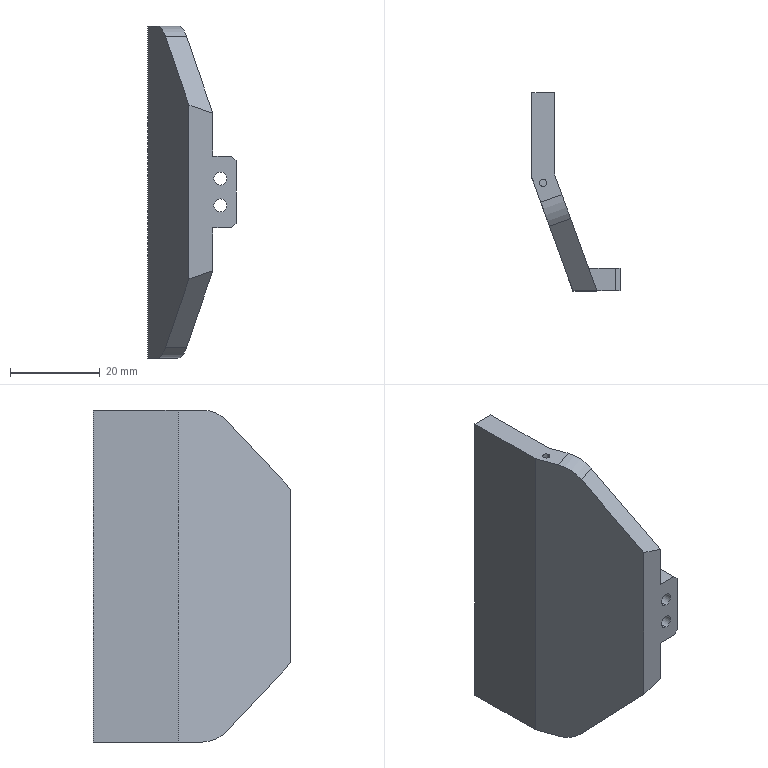NC program | NX | posted with a generic post | part box 19.643 x 44.061 x 74 mm
Lines 1 to 841 of 6515:
N10 G17 G21 G94 G90
(ADAPTIVE_MILLING_1 , TOOL : D8开粗)
N12 T02 M6
N14 G54
N16 G17 G0 G90 X47.519 Y39.467 B0. C0. S6500 M3
N18 G43 Z30. H2
N20 Z-18.35
N22 G94 G1 X47.451 Y39.6 Z-19.287 F3000.
N24 X47.383 Y39.734 Z-19.658
N26 X47.314 Y39.868 Z-19.93
N28 X47.246 Y40.001 Z-20.15
N30 X47.178 Y40.135 Z-20.334
N32 X47.109 Y40.268 Z-20.492
N34 X47.041 Y40.402 Z-20.63
N36 X46.972 Y40.535 Z-20.75
N38 X46.904 Y40.669 Z-20.855
N40 X46.836 Y40.802 Z-20.948
N42 X46.767 Y40.936 Z-21.029
N44 X46.699 Y41.069 Z-21.1
N46 X46.631 Y41.203 Z-21.16
N48 X46.562 Y41.336 Z-21.212
N50 X46.494 Y41.47 Z-21.255
N52 X46.426 Y41.603 Z-21.289
N54 X46.357 Y41.737 Z-21.316
N56 X46.289 Y41.87 Z-21.335
N58 X46.221 Y42.004 Z-21.346
N60 X46.152 Y42.138 Z-21.35
N62 X45.419 Y43.571
N64 G3 X43.987 Y43.584 R0.808
N66 G2 X43.689 Y42.483 R13.522
N68 G3 X43.278 Y38.319 R22.901
N70 X43.199 Y28.427 R395.024
N72 G1 X43.198 Y1.227
N74 G2 X41.595 Y-1.881 R4.329
N76 X37.82 Y-3.617 R8.394
N78 X32.452 Y-4.133 R29.955
N80 X22.352 Y-4.198 R519.939
N82 G1 X-37.82 Y-4.196
N84 G2 X-40.911 Y-2.558 R4.362
N86 X-42.627 Y1.228 R8.498
N88 X-43.134 Y6.597 R30.315
N90 X-43.199 Y16.596 R510.859
N92 G1 X-43.198 Y41.384
N94 G3 X-43.307 Y41.858 R1.202
N96 G1 X-43.582 Y42.28
N98 G2 X-43.965 Y43.549 R5.41
N100 G1 X-44.011 Y43.638
N102 G3 X-45.486 Y43.549 R0.808
N104 G1 X-45.765 Y42.801
N106 G3 X-45.725 Y42.146 R0.811
N108 G1 X-45.656 Y42.013 Z-21.346
N110 X-45.587 Y41.879 Z-21.335
N112 X-45.518 Y41.746 Z-21.316
N114 X-45.449 Y41.613 Z-21.289
N116 X-45.38 Y41.48 Z-21.255
N118 X-45.311 Y41.347 Z-21.212
N120 X-45.241 Y41.214 Z-21.16
N122 X-45.172 Y41.081 Z-21.1
N124 X-45.103 Y40.948 Z-21.029
N126 X-45.034 Y40.815 Z-20.948
N128 X-44.965 Y40.682 Z-20.855
N130 X-44.896 Y40.548 Z-20.75
N132 X-44.826 Y40.415 Z-20.63
N134 X-44.757 Y40.282 Z-20.492
N136 X-44.688 Y40.149 Z-20.334
N138 X-44.619 Y40.016 Z-20.15
N140 X-44.55 Y39.883 Z-19.93
N142 X-44.481 Y39.75 Z-19.658
N144 X-44.411 Y39.617 Z-19.287
N146 X-44.342 Y39.484 Z-18.35
N148 G0 Z30.
N150 X49.186 Y42.158
N152 Z-18.35
N154 G1 X49.036 Y42.157 Z-19.287
N156 X48.886 Y42.156 Z-19.658
N158 X48.736 Y42.155 Z-19.93
N160 X48.586 Y42.154 Z-20.15
N162 X48.436 Y42.153 Z-20.334
N164 X48.286 Y42.152 Z-20.492
N166 X48.136 Y42.151 Z-20.63
N168 X47.986 Y42.15 Z-20.75
N170 X47.836 Y42.149 Z-20.855
N172 X47.686 Y42.148 Z-20.948
N174 X47.536 Y42.147 Z-21.029
N176 X47.386 Y42.146 Z-21.1
N178 X47.236 Y42.145 Z-21.16
N180 X47.086 Y42.144 Z-21.212
N182 X46.936 Y42.143 Z-21.255
N184 X46.786 Y42.142 Z-21.289
N186 X46.636 Y42.141 Z-21.316
N188 X46.486 Y42.14 Z-21.335
N190 X46.336 Y42.139 Z-21.346
N192 X46.186 Y42.138 Z-21.35
N194 G2 X45.458 Y42.585 R0.809
N196 G1 X45.339 Y42.829
N198 X45.206 Y43.066
N200 G3 X43.792 Y42.864 R0.808
N202 G2 X43.35 Y41.852 R4.978
N204 G3 X42.658 Y38.601 R11.16
N206 X42.413 Y31.11 R91.281
N208 G1 X42.4 Y23.527
N210 X42.399 Y3.627
N212 G2 X39.878 Y-1.036 R5.88
N214 X35.46 Y-2.819 R10.805
N216 X29.489 Y-3.334 R37.58
N218 X21.889 Y-3.405 R624.145
N220 G3 X21.405 Y-3.619 R1.216
N222 G2 X19.349 Y-4.15 R4.218
N224 G1 X-19.35
N226 G2 X-20.963 Y-3.864 R6.112
N228 G3 X-25.268 Y-3.468 R24.879
N230 X-35.673 Y-3.385 R646.994
N232 G2 X-40.095 Y-0.795 R5.925
N234 X-41.819 Y3.542 R10.895
N236 X-42.339 Y9.713 R38.434
N238 X-42.398 Y20.113 R642.761
N240 G1 X-42.399 Y39.27
N242 G3 X-42.543 Y40.89 R5.724
N244 X-43.08 Y41.509 R2.07
N246 G1 X-43.352 Y41.928
N248 G3 X-44.446 Y42.171 R0.8
N250 X-44.827 Y41.505 Z-21.299 R0.832
N252 G1 X-44.914 Y40.737 Z-21.25
N254 X-45.121 Y38.865 F15000.
N256 Y11.851
N258 G3 X-44.506 Y5.031 R38.162
N260 G1 X-44.281 Y3.774
N262 X-44.038 Y2.522
N264 G3 X-42.742 Y-1.057 R14.501
N266 X-41.513 Y-2.978 R15.741
N268 X-40.029 Y-4.321 R5.81
N270 X-38.641 Y-5.034 R7.849
N272 X-36.99 Y-5.588 R11.3
N274 X-35.34 Y-5.823 R9.123
N276 G1 X-23.257 Y-6.413
N278 G3 X-22.886 Y-6.342 R0.84
N280 G1 X-21.535 Y-5.725
N282 X-21.089 Y-5.526 Z-21.281 F3000.
N284 X-20.65 Y-5.312 Z-21.312
N286 G3 X-20.312 Y-4.84 Z-21.35 R0.82
N288 X-20.756 Y-3.913 R0.8
N290 X-24.362 Y-2.902 R9.635
N292 X-31.396 Y-2.616 R73.042
N294 G2 X-34.381 Y-2.532 R27.551
N296 X-39.329 Y0.732 R6.952
N298 X-41.059 Y5.608 R12.894
N300 X-41.547 Y12.285 R47.439
N302 X-41.598 Y23.963 R752.767
N304 G1 X-41.599 Y37.464
N306 G3 X-41.764 Y39.951 R13.052
N308 X-42.415 Y40.872 R1.137
N310 G1 X-42.704 Y41.149
N312 G3 X-43.647 Y41.269 R0.8
N314 X-44.059 Y40.626 Z-21.3 R0.832
N316 G1 X-44.187 Y39.859 Z-21.25
N318 X-44.461 Y38.218 F15000.
N320 X-44.472 Y38.086
N322 Y16.966
N324 G3 X-43.847 Y8.17 R62.252
N326 G1 X-43.6 Y6.42
N328 X-43.337 Y4.672
N330 G3 X-42.42 Y1.478 R15.765
N332 X-41.535 Y-0.265 R13.083
N334 G1 X-41.071 Y-1.034
N336 X-40.594 Y-1.796
N338 G3 X-39.167 Y-3.193 R5.39
N340 X-37.794 Y-3.931 R7.292
N342 X-35.475 Y-4.691 R12.9
N344 X-33.784 Y-4.943 R16.452
N346 G1 X-32.686 Y-5.04
N348 X-31.586 Y-5.103
N350 X-24.47 Y-5.386
N352 X-24.347 Y-5.381
N354 X-22.622 Y-5.183
N356 X-22.129 Y-5.129 Z-21.282 F3000.
N358 X-21.639 Y-5.061 Z-21.313
N360 G3 X-21.177 Y-4.729 Z-21.35 R0.82
N362 X-21.408 Y-3.618 R0.8
N364 X-24.521 Y-2.342 R6.919
N366 X-30.258 Y-1.871 R38.181
N368 G2 X-33.43 Y-1.652 R18.825
N370 X-38.545 Y2.083 R7.687
N372 X-40.237 Y7.081 R14.105
N374 X-40.748 Y14.457 R51.567
N376 G1 X-40.782 Y16.924
N378 G2 X-41.15 Y19.692 R12.965
N380 G1 X-41.162 Y39.106
N382 G3 X-41.486 Y40.256 R2.241
N384 X-42.186 Y40.737 R2.579
N386 X-43.402 Y39.552 R0.88
N388 G1 X-42.8 Y38.466
N390 G3 X-41.15 Y38.892 R0.88
N392 X-41.174 Y39.802 R10.963
N394 X-41.738 Y40.473 R0.999
N396 X-42.541 Y40.479 R0.801
N398 X-42.884 Y40.125 Z-21.318 R1.067
N400 G1 X-43.509 Y39.252 Z-21.25
N402 X-44.089 Y38.444 F15000.
N404 G3 X-44.238 Y37.972 R0.81
N406 G1 X-44.218 Y34.372
N408 X-44.182 Y30.771
N410 G3 X-43.784 Y21.781 R167.581
N412 G1 X-42.839 Y8.553
N414 G3 X-42.083 Y4.147 R22.504
N416 X-40.552 Y0.638 R15.458
N418 X-38.707 Y-1.601 R8.256
N420 X-37.389 Y-2.616 R11.042
N422 X-34.887 Y-3.698 R8.477
N424 X-31.522 Y-4.34 R23.261
N426 G1 X-24.942 Y-5.078
N428 X-24.734 Y-5.074
N430 X-23.133 Y-4.834
N432 X-22.65 Y-4.765 Z-21.281 F3000.
N434 X-22.168 Y-4.68 Z-21.312
N436 G3 X-21.713 Y-4.32 Z-21.35 R0.82
N438 X-21.88 Y-3.31 R0.8
N440 X-24.557 Y-1.837 R5.524
N442 X-29.272 Y-1.184 R23.936
N444 G2 X-32.728 Y-0.745 R15.977
N446 X-37.791 Y3.379 R8.362
N448 X-39.464 Y8.697 R15.675
N450 X-39.912 Y14.476 R50.345
N452 G3 X-40.264 Y15.339 R4.186
N454 G2 X-40.786 Y16.945 R16.439
N456 G3 X-42.246 Y17.213 R0.8
N458 X-42.379 Y16.683 Z-21.315 R1.026
N460 G1 X-42.448 Y15.667 Z-21.25
N462 X-42.56 Y13.958 F15000.
N464 X-41.83 Y8.033
N466 G3 X-40.713 Y3.794 R16.281
N468 X-38.925 Y0.913 R11.255
N470 G1 X-38.185 Y0.043
N472 X-37.435 Y-0.818
N474 G3 X-36.179 Y-1.84 R6.318
N476 X-32.546 Y-3.249 R10.674
N478 G1 X-25.518 Y-4.57
N480 X-25.378 Y-4.581
N482 X-25.237 Y-4.572
N484 X-23.732 Y-4.318
N486 X-23.243 Y-4.239 Z-21.282 F3000.
N488 X-22.758 Y-4.145 Z-21.313
N490 G3 X-22.314 Y-3.789 Z-21.35 R0.82
N492 X-22.455 Y-2.801 R0.8
N494 X-25.136 Y-1.194 R5.529
N496 X-29.158 Y-0.477 R22.394
N498 G2 X-33.36 Y0.723 R11.126
N500 X-37.422 Y5.402 R9.596
N502 X-38.803 Y11.115 R19.758
N504 G3 X-39.012 Y13.042 R70.143
N506 X-39.529 Y13.873 R4.31
N508 G1 X-39.996 Y14.757
N510 G3 X-41.153 Y15.045 R0.8
N512 X-41.506 Y14.4 Z-21.302 R0.837
N514 G1 X-41.597 Y13.596 Z-21.25
N516 X-41.697 Y12.737 F15000.
N518 X-41.786 Y11.878
N520 X-41.764 Y11.694
N522 X-41.423 Y10.263
N524 X-41.053 Y8.84
N526 G3 X-40.003 Y5.496 R72.342
N528 X-38.576 Y2.468 R17.102
N530 G1 X-38.225 Y1.878
N532 X-37.861 Y1.296
N534 G3 X-35.899 Y-0.577 R6.875
N536 X-34.784 Y-1.184 R11.154
N538 X-32.058 Y-2.253 R15.897
N540 G1 X-26.173 Y-3.953
N542 G3 X-25.808 Y-3.971 R0.847
N544 G1 X-24.375 Y-3.711
N546 X-23.888 Y-3.625 Z-21.282 F3000.
N548 X-23.403 Y-3.525 Z-21.313
N550 G3 X-22.964 Y-3.163 Z-21.35 R0.82
N552 X-23.111 Y-2.185 R0.8
N554 X-24.692 Y-0.956 R6.119
N556 X-27.666 Y-0.037 R12.232
N558 G2 X-31.319 Y0.947 R18.853
N560 X-36.4 Y5.996 R9.853
N562 X-37.841 Y11.052 R18.99
N564 G3 X-38.117 Y11.998 R2.48
N566 G2 X-39.132 Y13.289 R7.463
N568 G3 X-40.523 Y13.168 R0.8
N570 X-40.564 Y12.611 Z-21.314 R0.862
N572 G1 X-40.373 Y11.627 Z-21.25
N574 X-40.051 Y9.95 F15000.
N576 X-40.039 Y9.138
N578 X-39.993 Y8.775
N580 X-39.912 Y8.418
N582 X-39.696 Y7.664
N584 X-39.47 Y6.912
N586 G3 X-38.559 Y4.749 R14.77
N588 G1 X-37.905 Y3.511
N590 G3 X-35.674 Y0.859 R10.163
N592 X-33.887 Y-0.402 R12.111
N594 X-30.813 Y-1.86 R17.553
N596 G1 X-26.902 Y-3.267
N598 G3 X-26.479 Y-3.3 R0.819
N600 G1 X-25.095 Y-3.033
N602 X-24.608 Y-2.943 Z-21.282 F3000.
N604 X-24.124 Y-2.837 Z-21.313
N606 G3 X-23.689 Y-2.472 Z-21.35 R0.82
N608 X-23.839 Y-1.499 R0.8
N610 X-25.435 Y-0.25 R6.401
N612 X-28.249 Y0.775 R18.414
N614 G2 X-32.669 Y3.037 R12.3
N616 X-36.099 Y8.243 R11.684
N618 G1 X-36.88 Y10.693
N620 X-37.017 Y10.901
N622 G2 X-38.142 Y12.027 R10.235
N624 G3 X-39.369 Y12.002 R0.8
N626 X-39.523 Y11.301 Z-21.303 R0.839
N628 G1 X-39.393 Y10.482 Z-21.25
N630 X-39.132 Y8.844 F15000.
N632 X-39.102 Y8.725
N634 X-39.058 Y8.612
N636 X-36.861 Y4.219
N638 G3 X-35.422 Y2.26 R7.557
N640 X-33.929 Y0.991 R13.387
N642 X-31.454 Y-0.587 R17.
N644 G1 X-27.63 Y-2.582
N646 G3 X-27.086 Y-2.654 R0.807
N648 G1 X-25.803 Y-2.369
N650 X-25.339 Y-2.268 Z-21.28 F3000.
N652 X-24.876 Y-2.157 Z-21.311
N654 G3 X-24.41 Y-1.773 Z-21.35 R0.8
N656 X-24.567 Y-0.814 R0.8
N658 X-26.179 Y0.49 R7.602
N660 X-29.142 Y1.923 R108.846
N662 G2 X-34.849 Y7.999 R11.985
N664 G3 X-35.523 Y9.48 R19.012
N666 G1 X-37.031 Y10.915
N668 G3 X-38.354 Y10.132 R0.8
N670 G1 X-38.271 Y9.929 Z-21.336
N672 X-38.161 Y9.739 Z-21.322
N674 X-37.599 Y8.757 Z-21.25
N676 X-37.355 Y8.326 F15000.
N678 X-37.101 Y7.901
N680 X-37.031 Y7.821
N682 X-28.357 Y-0.861
N684 G3 X-27.937 Y-1.082 R0.812
N686 G1 X-26.97 Y-1.261
N688 X-25.998 Y-1.436 Z-21.313 F3000.
N690 G3 X-25.447 Y-1.29 Z-21.35 R0.801
N692 X-25.368 Y-0.06 R0.8
N694 X-27.593 Y1.771 R12.794
N696 G2 X-31.079 Y4.403 R20.895
N698 X-33.45 Y7.525 R14.751
N700 G1 X-35.624 Y9.591
N702 G3 X-36.945 Y8.803 R0.8
N704 G1 X-36.862 Y8.602 Z-21.336
N706 X-36.753 Y8.413 Z-21.322
N708 X-36.188 Y7.429 Z-21.25
N710 X-35.944 Y6.998 F15000.
N712 X-35.69 Y6.573
N714 X-35.624 Y6.496
N716 X-29.377 Y0.098
N718 G3 X-28.948 Y-0.13 R0.811
N720 G1 X-27.987 Y-0.305
N722 X-27.015 Y-0.477 Z-21.313 F3000.
N724 G3 X-26.464 Y-0.329 Z-21.35 R0.801
N726 X-26.388 Y0.899 R0.8
N728 G1 X-33.634 Y7.7
N730 X-34.705 Y8.183
N732 G3 X-35.583 Y6.854 R0.808
N734 G1 X-35.473 Y6.751 Z-21.346
N736 X-35.364 Y6.649 Z-21.335
N738 X-35.255 Y6.546 Z-21.316
N740 X-35.146 Y6.443 Z-21.289
N742 X-35.036 Y6.34 Z-21.255
N744 X-34.927 Y6.237 Z-21.212
N746 X-34.818 Y6.135 Z-21.16
N748 X-34.709 Y6.032 Z-21.1
N750 X-34.6 Y5.929 Z-21.029
N752 X-34.49 Y5.826 Z-20.948
N754 X-34.381 Y5.723 Z-20.855
N756 X-34.272 Y5.621 Z-20.75
N758 X-34.163 Y5.518 Z-20.63
N760 X-34.053 Y5.415 Z-20.492
N762 X-33.944 Y5.312 Z-20.334
N764 X-33.835 Y5.209 Z-20.15
N766 X-33.726 Y5.107 Z-19.93
N768 X-33.616 Y5.004 Z-19.658
N770 X-33.507 Y4.901 Z-19.287
N772 X-33.398 Y4.798 Z-18.35
N774 G0 Z30.
N776 X44.598 Y39.307
N778 Z-18.35
N780 G1 X44.649 Y39.448 Z-19.287
N782 X44.7 Y39.589 Z-19.658
N784 X44.751 Y39.731 Z-19.93
N786 X44.802 Y39.872 Z-20.15
N788 X44.853 Y40.013 Z-20.334
N790 X44.904 Y40.154 Z-20.492
N792 X44.954 Y40.295 Z-20.63
N794 X45.005 Y40.436 Z-20.75
N796 X45.056 Y40.577 Z-20.855
N798 X45.107 Y40.718 Z-20.948
N800 X45.158 Y40.859 Z-21.029
N802 X45.209 Y41.001 Z-21.1
N804 X45.26 Y41.142 Z-21.16
N806 X45.311 Y41.283 Z-21.212
N808 X45.361 Y41.424 Z-21.255
N810 X45.412 Y41.565 Z-21.289
N812 X45.463 Y41.706 Z-21.316
N814 X45.514 Y41.847 Z-21.335
N816 X45.565 Y41.988 Z-21.346
N818 X45.616 Y42.129 Z-21.35
N820 G3 X44.286 Y42.976 R0.808
N822 G1 X43.527 Y42.197
N824 G3 X42.578 Y40.522 R8.031
N826 X41.827 Y36.37 R15.953
N828 X41.608 Y27.218 R136.803
N830 G1 X41.6 Y20.027
N832 X41.599 Y5.727
N834 G2 X38.274 Y-0.325 R6.951
N836 X33.397 Y-2.059 R12.851
N838 X26.721 Y-2.547 R47.452
N840 G3 X23.171 Y-2.623 R97.012
N842 X22.377 Y-2.848 R1.502
N844 G2 X21.542 Y-3.53 R3.588
N846 G3 X21.299 Y-4.623 R0.8
N848 X21.965 Y-5.004 Z-21.299 R0.832
N850 G1 X22.733 Y-5.091 Z-21.25
N852 X24.605 Y-5.298 F15000.
N854 X25.914 Y-5.299
N856 X27.223 Y-5.289
N858 G3 X30.472 Y-4.975 R23.904
N860 G1 X32.248 Y-4.683
N862 X34.022 Y-4.374
N864 G3 X37.172 Y-3.522 R23.281
N866 G1 X37.821 Y-3.297
N868 X38.466 Y-3.062
N870 G3 X41.034 Y-1.327 R7.27
N872 G1 X41.757 Y-0.479
N874 X42.46 Y0.385
N876 G3 X43.526 Y2.66 R6.369
N878 X43.916 Y5.558 R13.92
N880 G1 X44.846 Y38.524
N882 X44.566 Y40.209
N884 X44.488 Y40.695 Z-21.281 F3000.
N886 X44.394 Y41.178 Z-21.313
N888 G3 X44.032 Y41.624 Z-21.35 R0.82
N890 X43.08 Y41.509 R0.8
N892 X41.855 Y39.584 R4.204
N894 X41.15 Y36.15 R15.621
N896 G1 X41.148 Y19.547
N898 G2 X40.934 Y16.84 R136.048
N900 G3 X40.793 Y7.226 R226.74
N902 G2 X36.865 Y0.429 R7.693
N904 X31.868 Y-1.245 R14.209
N906 X25.348 Y-1.74 R50.712
N908 G3 X23.428 Y-1.959 R8.858
N910 G1 X23.194 Y-2.09
N912 X22.314 Y-2.907
N914 G3 X22.156 Y-3.876 R0.8
N916 X22.806 Y-4.295 Z-21.299 R0.831
N918 G1 X23.562 Y-4.418 Z-21.25
N920 X25.136 Y-4.673 F15000.
N922 X25.256 Y-4.681
N924 X25.377 Y-4.675
N926 X31.211 Y-3.841
N928 G3 X35.567 Y-2.819 R25.097
N930 X38.968 Y-1.19 R15.761
N932 X41.341 Y1.247 R8.111
N934 G1 X41.707 Y1.829
N936 X42.062 Y2.417
N938 G3 X42.858 Y4.607 R7.816
N940 G1 X42.96 Y5.184
N942 X43.028 Y5.766
N944 G3 X43.347 Y10.662 R96.5
N946 G1 X43.533 Y15.631
N948 X43.52 Y15.796
N950 X43.477 Y15.955
N952 X42.903 Y17.41
N954 X42.534 Y18.332 Z-21.313 F3000.
N956 G3 X42.123 Y18.72 Z-21.35 R0.801
N958 X41.032 Y18.132 R0.8
N960 G2 X40.528 Y15.997 R14.344
N962 G3 X40.09 Y11.709 R23.887
N964 G2 X39.951 Y7.773 R86.837
N966 X35.597 Y1.212 R8.225
N968 X30.285 Y-0.464 R15.511
N970 X25.532 Y-0.926 R79.885
N972 G3 X24.255 Y-1.163 R6.098
N974 G1 X24.08 Y-1.268
N976 X23.127 Y-2.152
N978 G3 X22.967 Y-3.118 R0.8
N980 X23.615 Y-3.54 Z-21.299 R0.831
N982 G1 X24.371 Y-3.667 Z-21.25
N984 X25.185 Y-3.806 F15000.
N986 X26. Y-3.934
N988 X26.19 Y-3.92
N990 X29.077 Y-3.349
N992 G3 X31.933 Y-2.643 R51.411
N994 G1 X33.352 Y-2.25
N996 X34.768 Y-1.841
N998 G3 X38.207 Y-0.032 R11.23
N1000 X39.287 Y0.954 R10.436
N1002 G1 X39.906 Y1.605
N1004 X40.515 Y2.266
N1006 G3 X41.5 Y4.007 R5.767
N1008 X42.017 Y5.993 R11.423
N1010 X42.48 Y8.899 R45.097
N1012 G1 X43.077 Y13.691
N1014 G3 X43.017 Y14.108 R0.82
N1016 G1 X42.424 Y15.476
N1018 X42.231 Y15.933 Z-21.282 F3000.
N1020 X42.023 Y16.383 Z-21.313
N1022 G3 X41.573 Y16.728 Z-21.35 R0.82
N1024 X40.576 Y16.192 R0.8
N1026 G2 X40.084 Y14.935 R8.328
N1028 G3 X39.419 Y11.353 R13.428
N1030 G2 X39.009 Y7.818 R24.146
N1032 X34.451 Y2.016 R8.792
N1034 X29.22 Y0.378 R16.369
N1036 G3 X25.668 Y-0.14 R112.702
N1038 X24.683 Y-0.709 R1.579
N1040 G1 X24.023 Y-1.321
N1042 G3 X23.859 Y-2.28 R0.8
N1044 X24.5 Y-2.708 Z-21.299 R0.831
N1046 G1 X25.256 Y-2.845 Z-21.25
N1048 X26.713 Y-3.11 F15000.
N1050 G3 X27.085 Y-3.089 R0.843
N1052 G1 X31.32 Y-1.822
N1054 G3 X35.827 Y0.061 R23.293
N1056 G1 X36.441 Y0.397
N1058 X37.049 Y0.742
N1060 G3 X39.267 Y2.722 R8.464
N1062 X40.567 Y4.782 R10.906
N1064 X41.387 Y6.834 R11.252
N1066 X41.723 Y8.955 R9.596
N1068 G1 X41.852 Y11.873
N1070 X41.85 Y11.98
N1072 X41.69 Y13.74
N1074 X41.595 Y14.733 Z-21.314 F3000.
N1076 G3 X41.315 Y15.218 Z-21.35 R0.802
N1078 X40.084 Y14.935 R0.8
N1080 X39.304 Y13.299 R19.956
N1082 X38.621 Y10.163 R21.823
N1084 G2 X36.735 Y5.585 R10.392
N1086 X31.734 Y2.099 R10.788
N1088 X27.305 Y0.994 R30.864
N1090 G3 X26.205 Y0.692 R5.286
N1092 X25.005 Y-0.405 R15.085
N1094 X25.043 Y-1.604 R0.8
N1096 X25.757 Y-1.765 Z-21.302 R0.837
N1098 G1 X26.559 Y-1.632 Z-21.25
N1100 X28.421 Y-1.321 F15000.
N1102 X29.898 Y-0.953
N1104 X31.372 Y-0.573
N1106 G3 X35.146 Y1.035 R16.228
N1108 X37.263 Y2.602 R12.449
N1110 X38.571 Y4.054 R13.047
N1112 X40.36 Y7.465 R9.74
N1114 G1 X41.374 Y10.935
N1116 X41.402 Y11.098
N1118 X41.399 Y11.264
N1120 X41.193 Y12.826
N1122 X41.133 Y13.314 Z-21.281 F3000.
N1124 X41.057 Y13.799 Z-21.313
N1126 G3 X40.71 Y14.259 Z-21.35 R0.82
N1128 X39.605 Y13.998 R0.8
N1130 X38.199 Y11.055 R8.688
N1132 G2 X36.558 Y7.272 R14.672
N1134 X31.352 Y3.147 R11.053
N1136 X27.649 Y1.95 R43.429
N1138 G1 X27.348 Y1.796
N1140 X26.036 Y0.563
N1142 G3 X26.102 Y-0.658 R0.8
N1144 X26.81 Y-0.791 Z-21.303 R0.838
N1146 G1 X27.621 Y-0.633 Z-21.25
N1148 X28.183 Y-0.527 F15000.
N1150 X28.741 Y-0.407
N1152 X28.891 Y-0.336
N1154 X29.025 Y-0.237
N1156 X40.59 Y10.474
N1158 G3 X40.829 Y11.223 R0.801
N1160 G1 X40.663 Y12.027
N1162 X40.568 Y12.506 Z-21.281 F3000.
N1164 X40.457 Y12.983 Z-21.312
N1166 G3 X40.073 Y13.417 Z-21.35 R0.82
N1168 X39.042 Y13.154 R0.8
N1170 G2 X38.319 Y12.18 R14.261
N1172 G3 X36.885 Y9.567 R45.43
N1174 G2 X34.583 Y6.542 R12.574
N1176 G1 X31.247 Y3.426
N1178 G2 X30.402 Y3.246 R2.377
N1180 G3 X28.569 Y2.87 R12.933
N1182 G1 X28.364 Y2.751
N1184 X27.344 Y1.792
N1186 G3 X27.405 Y0.574 R0.8
N1188 X28.116 Y0.437 Z-21.302 R0.838
N1190 G1 X28.923 Y0.593 Z-21.25
N1192 X29.485 Y0.697 F15000.
N1194 X30.044 Y0.817
N1196 X30.197 Y0.89
N1198 X30.333 Y0.991
N1200 X39.338 Y9.486
N1202 G3 X39.576 Y9.922 R0.81
N1204 G1 X39.752 Y10.869
N1206 X39.931 Y11.862 Z-21.314 F3000.
N1208 G3 X39.798 Y12.396 Z-21.35 R0.802
N1210 X38.538 Y12.474 R0.8
N1212 X35.814 Y9.238 R43.803
N1214 G2 X31.615 Y4.964 R42.409
N1216 G1 X30.041 Y4.3
N1218 G3 X28.342 Y2.73 R32.979
N1220 X28.405 Y1.511 R0.8
N1222 X29.116 Y1.376 Z-21.302 R0.838
N1224 G1 X29.923 Y1.533 Z-21.25
N1226 X30.487 Y1.64 F15000.
N1228 X31.048 Y1.761
N1230 X31.198 Y1.831
N1232 X31.331 Y1.929
N1234 X38.373 Y8.419
N1236 G3 X38.62 Y8.876 R0.808
N1238 G1 X38.783 Y9.85
N1240 X38.868 Y10.337 Z-21.282 F3000.
N1242 X38.938 Y10.827 Z-21.313
N1244 G3 X38.746 Y11.363 Z-21.35 R0.82
N1246 X37.572 Y11.408 R0.8
N1248 G1 X37.468 Y11.305
N1250 X34.93 Y8.92
N1252 X29.901 Y4.195
N1254 G3 X30.56 Y2.82 R0.8
N1256 G1 X30.756 Y2.875 Z-21.337
N1258 X30.939 Y2.961 Z-21.324
N1260 X31.986 Y3.472 Z-21.25
N1262 X33.375 Y4.152 F15000.
N1264 X34.232 Y4.79
N1266 X35.08 Y5.44
N1268 G3 X36.797 Y7.044 R16.528
N1270 G1 X38.334 Y8.699
N1272 X39.861 Y10.363
N1274 G3 X41.569 Y12.631 R19.052
N1276 X42.804 Y15.388 R11.574
N1278 X43.303 Y17.678 R14.65
N1280 X43.576 Y20.606 R36.704
N1282 G1 X44.487 Y38.1
N1284 X44.477 Y38.276
N1286 X44.208 Y39.852
N1288 X44.131 Y40.32 Z-21.28 F3000.
N1290 X44.043 Y40.786 Z-21.31
N1292 G3 X43.682 Y41.272 Z-21.35 R0.8
N1294 X42.719 Y41.163 R0.8
N1296 X41.159 Y38.815 R4.763
N1298 G1 X41.15 Y36.15
N1300 G3 X42.66 Y35.535 R0.88
N1302 X42.922 Y36.119 Z-21.309 R1.055
N1304 G1 X43.111 Y37.019 Z-21.25
N1306 X43.587 Y39.284 F15000.
N1308 X43.671 Y39.672 Z-21.275 F3000.
N1310 X43.74 Y40.062 Z-21.3
N1312 G3 X43.459 Y40.761 Z-21.35 R0.892
N1314 X42.415 Y40.872 R0.88
N1316 X41.202 Y39.719 R2.598
N1318 G1 X41.15 Y39.491
N1320 Y38.691
N1322 G3 X42.862 Y38.406 R0.88
N1324 G1 X43.263 Y39.574
N1326 G3 X41.984 Y40.618 R0.88
N1328 X41.296 Y40.1 R1.892
N1330 X41.15 Y39.395 R1.23
N1332 X41.979 Y38.587 R0.808
N1334 G1 X43.115 Y38.616
N1336 X43.264 Y38.619 Z-21.346
N1338 X43.414 Y38.623 Z-21.335
N1340 X43.564 Y38.627 Z-21.316
N1342 X43.714 Y38.631 Z-21.289
N1344 X43.864 Y38.635 Z-21.255
N1346 X44.014 Y38.639 Z-21.212
N1348 X44.164 Y38.642 Z-21.16
N1350 X44.314 Y38.646 Z-21.1
N1352 X44.464 Y38.65 Z-21.029
N1354 X44.614 Y38.654 Z-20.948
N1356 X44.764 Y38.658 Z-20.855
N1358 X44.914 Y38.662 Z-20.75
N1360 X45.064 Y38.665 Z-20.63
N1362 X45.214 Y38.669 Z-20.492
N1364 X45.364 Y38.673 Z-20.334
N1366 X45.514 Y38.677 Z-20.15
N1368 X45.664 Y38.681 Z-19.93
N1370 X45.814 Y38.684 Z-19.658
N1372 X45.964 Y38.688 Z-19.287
N1374 X46.114 Y38.692 Z-18.35
N1376 G0 Z30.
N1378 X-41.805 Y8.712
N1380 Z-12.885
N1382 G1 X-41.701 Y8.82 Z-13.822
N1384 X-41.596 Y8.927 Z-14.193
N1386 X-41.492 Y9.035 Z-14.465
N1388 X-41.387 Y9.143 Z-14.685
N1390 X-41.283 Y9.25 Z-14.869
N1392 X-41.178 Y9.358 Z-15.028
N1394 X-41.074 Y9.466 Z-15.165
N1396 X-40.969 Y9.573 Z-15.285
N1398 X-40.865 Y9.681 Z-15.391
N1400 X-40.76 Y9.788 Z-15.483
N1402 X-40.656 Y9.896 Z-15.564
N1404 X-40.551 Y10.004 Z-15.635
N1406 X-40.447 Y10.111 Z-15.695
N1408 X-40.342 Y10.219 Z-15.747
N1410 X-40.238 Y10.327 Z-15.79
N1412 X-40.133 Y10.434 Z-15.824
N1414 X-40.029 Y10.542 Z-15.851
N1416 X-39.924 Y10.649 Z-15.87
N1418 X-39.82 Y10.757 Z-15.881
N1420 X-39.715 Y10.865 Z-15.885
N1422 X-38.819 Y11.788
N1424 G3 X-38.733 Y12.807 R0.808
N1426 G1 X-39.356 Y13.717
N1428 G2 X-40.338 Y15.827 R19.747
N1430 X-40.956 Y18.315 R14.315
N1432 G3 X-41.752 Y18.982 R0.808
N1434 G1 X-43.029 Y18.981
N1436 X-43.179 Z-15.881
N1438 X-43.329 Z-15.87
N1440 X-43.479 Z-15.851
N1442 X-43.629 Z-15.824
N1444 X-43.779 Z-15.79
N1446 X-43.929 Z-15.747
N1448 X-44.079 Y18.98 Z-15.695
N1450 X-44.229 Z-15.635
N1452 X-44.379 Z-15.564
N1454 X-44.529 Z-15.483
N1456 X-44.679 Z-15.391
N1458 X-44.829 Z-15.285
N1460 X-44.979 Z-15.165
N1462 X-45.129 Z-15.028
N1464 X-45.279 Z-14.869
N1466 X-45.429 Y18.979 Z-14.685
N1468 X-45.579 Z-14.465
N1470 X-45.729 Z-14.193
N1472 X-45.879 Z-13.822
N1474 X-46.029 Z-12.885
N1476 G0 Z30.
N1478 X-39.805 Y6.711
N1480 Z-12.388
N1482 G1 X-39.708 Y6.825 Z-13.325
N1484 X-39.611 Y6.94 Z-13.696
N1486 X-39.514 Y7.054 Z-13.969
N1488 X-39.417 Y7.168 Z-14.188
N1490 X-39.32 Y7.283 Z-14.373
N1492 X-39.223 Y7.397 Z-14.531
N1494 X-39.126 Y7.511 Z-14.668
N1496 X-39.029 Y7.626 Z-14.788
N1498 X-38.932 Y7.74 Z-14.894
N1500 X-38.835 Y7.855 Z-14.986
N1502 X-38.738 Y7.969 Z-15.067
N1504 X-38.641 Y8.083 Z-15.138
N1506 X-38.543 Y8.198 Z-15.199
N1508 X-38.446 Y8.312 Z-15.25
N1510 X-38.349 Y8.427 Z-15.293
N1512 X-38.252 Y8.541 Z-15.328
N1514 X-38.155 Y8.655 Z-15.354
N1516 X-38.058 Y8.77 Z-15.373
N1518 X-37.961 Y8.884 Z-15.385
N1520 X-37.864 Y8.999 Z-15.388
N1522 X-37.07 Y9.936
N1524 G3 X-37.097 Y11.012 R0.808
N1526 G2 X-39.951 Y15.046 R14.72
N1528 X-40.936 Y18.288 R14.296
N1530 G3 X-41.74 Y18.949 R0.808
N1532 G1 X-43.014 Y18.934
N1534 X-43.164 Y18.933 Z-15.385
N1536 X-43.314 Y18.931 Z-15.373
N1538 X-43.464 Y18.929 Z-15.354
N1540 X-43.614 Y18.927 Z-15.328
N1542 X-43.764 Y18.926 Z-15.293
N1544 X-43.914 Y18.924 Z-15.25
N1546 X-44.064 Y18.922 Z-15.199
N1548 X-44.214 Y18.921 Z-15.138
N1550 X-44.364 Y18.919 Z-15.067
N1552 X-44.514 Y18.917 Z-14.986
N1554 X-44.664 Y18.916 Z-14.894
N1556 X-44.814 Y18.914 Z-14.788
N1558 X-44.964 Y18.912 Z-14.668
N1560 X-45.114 Y18.91 Z-14.531
N1562 X-45.264 Y18.909 Z-14.373
N1564 X-45.414 Y18.907 Z-14.188
N1566 X-45.564 Y18.905 Z-13.969
N1568 X-45.714 Y18.904 Z-13.696
N1570 X-45.864 Y18.902 Z-13.325
N1572 X-46.014 Y18.9 Z-12.388
N1574 G0 Z30.
N1576 X-38.096 Y5.128
N1578 Z-11.891
N1580 G1 X-38.007 Y5.249 Z-12.828
N1582 X-37.918 Y5.369 Z-13.199
N1584 X-37.828 Y5.49 Z-13.472
N1586 X-37.739 Y5.61 Z-13.691
N1588 X-37.65 Y5.731 Z-13.876
N1590 X-37.561 Y5.852 Z-14.034
N1592 X-37.472 Y5.972 Z-14.171
N1594 X-37.383 Y6.093 Z-14.291
N1596 X-37.293 Y6.213 Z-14.397
N1598 X-37.204 Y6.334 Z-14.49
N1600 X-37.115 Y6.455 Z-14.571
N1602 X-37.026 Y6.575 Z-14.641
N1604 X-36.937 Y6.696 Z-14.702
N1606 X-36.848 Y6.817 Z-14.753
N1608 X-36.758 Y6.937 Z-14.796
N1610 X-36.669 Y7.058 Z-14.831
N1612 X-36.58 Y7.178 Z-14.858
N1614 X-36.491 Y7.299 Z-14.876
N1616 X-36.402 Y7.42 Z-14.888
N1618 X-36.313 Y7.54 Z-14.891
N1620 X-35.548 Y8.575
N1622 G3 X-35.609 Y9.609 R0.808
N1624 G1 X-37.678 Y11.811
N1626 G2 X-40.17 Y15.733 R14.217
N1628 G1 X-40.672 Y17.206
N1630 X-40.79 Y17.794
N1632 G3 X-41.637 Y18.442 R0.808
N1634 G1 X-42.906 Y18.356
N1636 X-43.055 Y18.346 Z-14.888
N1638 X-43.205 Y18.336 Z-14.876
N1640 X-43.355 Y18.326 Z-14.858
N1642 X-43.504 Y18.315 Z-14.831
N1644 X-43.654 Y18.305 Z-14.796
N1646 X-43.804 Y18.295 Z-14.753
N1648 X-43.953 Y18.285 Z-14.702
N1650 X-44.103 Y18.275 Z-14.641
N1652 X-44.253 Y18.265 Z-14.571
N1654 X-44.402 Y18.254 Z-14.49
N1656 X-44.552 Y18.244 Z-14.397
N1658 X-44.702 Y18.234 Z-14.291
N1660 X-44.851 Y18.224 Z-14.171
N1662 X-45.001 Y18.214 Z-14.034
N1664 X-45.151 Y18.204 Z-13.876
N1666 X-45.3 Y18.194 Z-13.691
N1668 X-45.45 Y18.183 Z-13.472
N1670 X-45.6 Y18.173 Z-13.199
N1672 X-45.749 Y18.163 Z-12.828
N1674 X-45.899 Y18.153 Z-11.891
N1676 G0 Z30.
N1678 X-36.767 Y3.884
N1680 Z-11.395